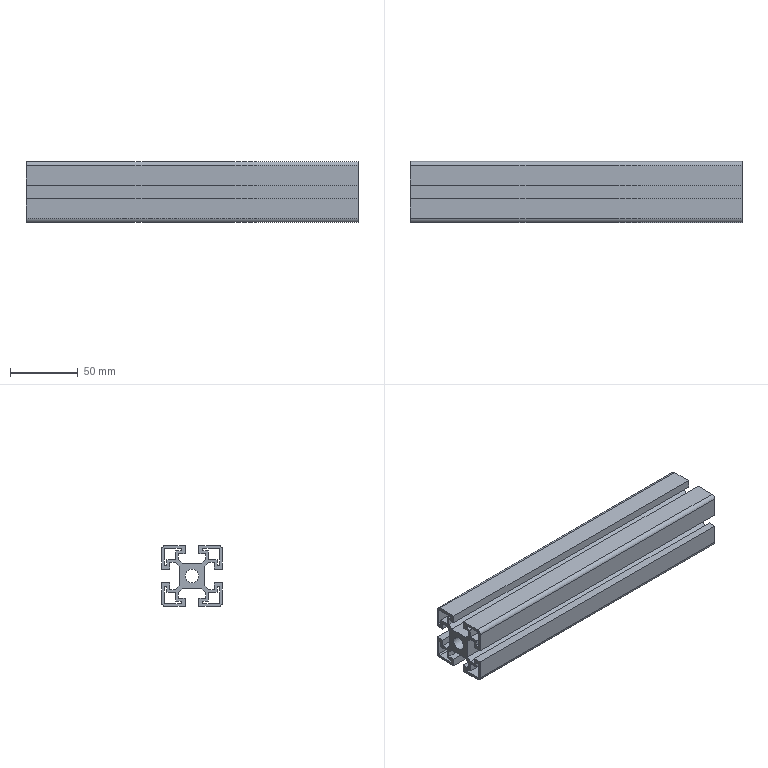Part | STEP file | 1_8 | 1 solid | 87 faces | box 245 x 45 x 45 mm | volume 200347 mm3 | plane 78 | cylinder 9 | commonest cylinder face diameters 2 x4 6 x4 10 x1